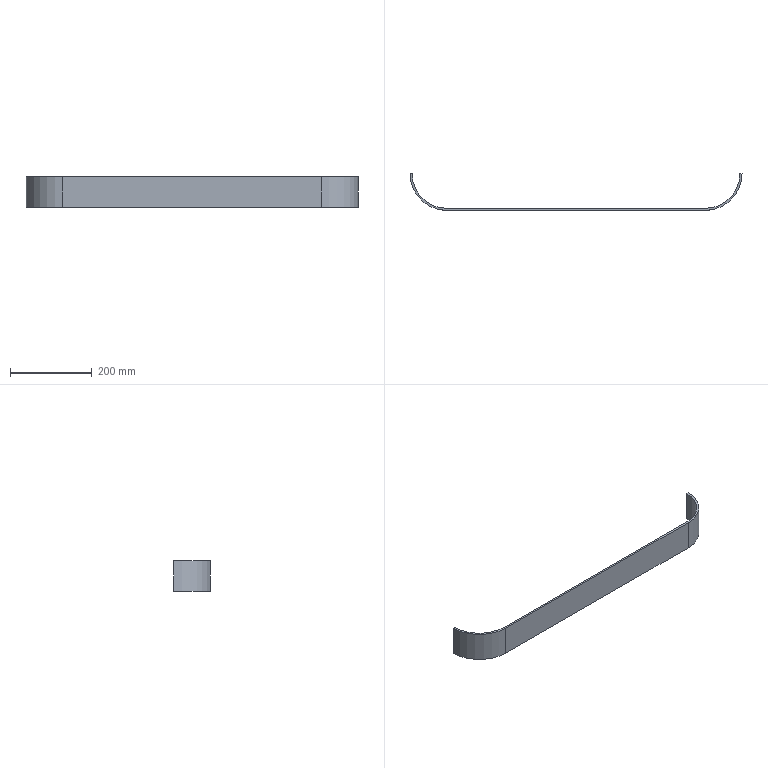Part | NX | features BREP 1 | 1 solid | 10 faces | box 810 x 90 x 75 mm | volume 339334 mm3 | plane 6 | cylinder 4 | commonest cylinder face diameters 170 x2 180 x2
STEP:
#1=CARTESIAN_POINT('',(-315.,0.,75.));
#2=VERTEX_POINT('',#1);
#3=CARTESIAN_POINT('',(-405.,90.,75.));
#4=VERTEX_POINT('',#3);
#5=CARTESIAN_POINT('',(-315.,90.,75.));
#6=DIRECTION('',(0.,0.,-1.));
#7=DIRECTION('',(-1.,0.,0.));
#8=AXIS2_PLACEMENT_3D('',#5,#6,#7);
#9=CIRCLE('',#8,90.);
#10=EDGE_CURVE('',#2,#4,#9,.T.);
#11=ORIENTED_EDGE('',*,*,#10,.F.);
#12=CARTESIAN_POINT('',(315.,0.,75.));
#13=VERTEX_POINT('',#12);
#14=CARTESIAN_POINT('',(-315.,0.,75.));
#15=DIRECTION('',(-1.,0.,0.));
#16=VECTOR('',#15,1000.);
#17=LINE('',#14,#16);
#18=EDGE_CURVE('',#13,#2,#17,.T.);
#19=ORIENTED_EDGE('',*,*,#18,.F.);
#20=CARTESIAN_POINT('',(405.,90.,75.));
#21=VERTEX_POINT('',#20);
#22=CARTESIAN_POINT('',(315.,90.,75.));
#23=DIRECTION('',(0.,0.,-1.));
#24=DIRECTION('',(-1.,0.,0.));
#25=AXIS2_PLACEMENT_3D('',#22,#23,#24);
#26=CIRCLE('',#25,90.);
#27=EDGE_CURVE('',#21,#13,#26,.T.);
#28=ORIENTED_EDGE('',*,*,#27,.F.);
#29=CARTESIAN_POINT('',(400.,90.,75.));
#30=VERTEX_POINT('',#29);
#31=CARTESIAN_POINT('',(400.,90.,75.));
#32=DIRECTION('',(1.,0.,0.));
#33=VECTOR('',#32,1000.);
#34=LINE('',#31,#33);
#35=EDGE_CURVE('',#30,#21,#34,.T.);
#36=ORIENTED_EDGE('',*,*,#35,.F.);
#37=CARTESIAN_POINT('',(315.,5.,75.));
#38=VERTEX_POINT('',#37);
#39=CARTESIAN_POINT('',(315.,90.,75.));
#40=DIRECTION('',(0.,0.,-1.));
#41=DIRECTION('',(1.,0.,0.));
#42=AXIS2_PLACEMENT_3D('',#39,#40,#41);
#43=CIRCLE('',#42,85.);
#44=EDGE_CURVE('',#30,#38,#43,.T.);
#45=ORIENTED_EDGE('',*,*,#44,.T.);
#46=CARTESIAN_POINT('',(-315.,5.,75.));
#47=VERTEX_POINT('',#46);
#48=CARTESIAN_POINT('',(-315.,5.,75.));
#49=DIRECTION('',(-1.,0.,0.));
#50=VECTOR('',#49,1000.);
#51=LINE('',#48,#50);
#52=EDGE_CURVE('',#38,#47,#51,.T.);
#53=ORIENTED_EDGE('',*,*,#52,.T.);
#54=CARTESIAN_POINT('',(-400.,90.,75.));
#55=VERTEX_POINT('',#54);
#56=CARTESIAN_POINT('',(-315.,90.,75.));
#57=DIRECTION('',(0.,0.,-1.));
#58=DIRECTION('',(1.,0.,0.));
#59=AXIS2_PLACEMENT_3D('',#56,#57,#58);
#60=CIRCLE('',#59,85.);
#61=EDGE_CURVE('',#47,#55,#60,.T.);
#62=ORIENTED_EDGE('',*,*,#61,.T.);
#63=CARTESIAN_POINT('',(-405.,90.,75.));
#64=DIRECTION('',(1.,0.,0.));
#65=VECTOR('',#64,1000.);
#66=LINE('',#63,#65);
#67=EDGE_CURVE('',#4,#55,#66,.T.);
#68=ORIENTED_EDGE('',*,*,#67,.F.);
#69=EDGE_LOOP('',(#11,#19,#28,#36,#45,#53,#62,#68));
#70=FACE_BOUND('',#69,.T.);
#71=CARTESIAN_POINT('',(-315.,5.,75.));
#72=DIRECTION('',(0.,0.,1.));
#73=DIRECTION('',(1.,0.,0.));
#74=AXIS2_PLACEMENT_3D('',#71,#72,#73);
#75=PLANE('',#74);
#76=ADVANCED_FACE('',(#70),#75,.T.);
#77=CARTESIAN_POINT('',(-315.,5.,0.));
#78=VERTEX_POINT('',#77);
#79=CARTESIAN_POINT('',(-400.,90.,0.));
#80=VERTEX_POINT('',#79);
#81=CARTESIAN_POINT('',(-315.,90.,0.));
#82=DIRECTION('',(0.,0.,-1.));
#83=DIRECTION('',(1.,0.,0.));
#84=AXIS2_PLACEMENT_3D('',#81,#82,#83);
#85=CIRCLE('',#84,85.);
#86=EDGE_CURVE('',#78,#80,#85,.T.);
#87=ORIENTED_EDGE('',*,*,#86,.F.);
#88=CARTESIAN_POINT('',(315.,5.,0.));
#89=VERTEX_POINT('',#88);
#90=CARTESIAN_POINT('',(-315.,5.,0.));
#91=DIRECTION('',(-1.,0.,0.));
#92=VECTOR('',#91,1000.);
#93=LINE('',#90,#92);
#94=EDGE_CURVE('',#89,#78,#93,.T.);
#95=ORIENTED_EDGE('',*,*,#94,.F.);
#96=CARTESIAN_POINT('',(400.,90.,0.));
#97=VERTEX_POINT('',#96);
#98=CARTESIAN_POINT('',(315.,90.,0.));
#99=DIRECTION('',(0.,0.,-1.));
#100=DIRECTION('',(1.,0.,0.));
#101=AXIS2_PLACEMENT_3D('',#98,#99,#100);
#102=CIRCLE('',#101,85.);
#103=EDGE_CURVE('',#97,#89,#102,.T.);
#104=ORIENTED_EDGE('',*,*,#103,.F.);
#105=CARTESIAN_POINT('',(405.,90.,0.));
#106=VERTEX_POINT('',#105);
#107=CARTESIAN_POINT('',(400.,90.,0.));
#108=DIRECTION('',(1.,0.,0.));
#109=VECTOR('',#108,1000.);
#110=LINE('',#107,#109);
#111=EDGE_CURVE('',#97,#106,#110,.T.);
#112=ORIENTED_EDGE('',*,*,#111,.T.);
#113=CARTESIAN_POINT('',(315.,0.,0.));
#114=VERTEX_POINT('',#113);
#115=CARTESIAN_POINT('',(315.,90.,0.));
#116=DIRECTION('',(0.,0.,-1.));
#117=DIRECTION('',(-1.,0.,0.));
#118=AXIS2_PLACEMENT_3D('',#115,#116,#117);
#119=CIRCLE('',#118,90.);
#120=EDGE_CURVE('',#106,#114,#119,.T.);
#121=ORIENTED_EDGE('',*,*,#120,.T.);
#122=CARTESIAN_POINT('',(-315.,0.,0.));
#123=VERTEX_POINT('',#122);
#124=CARTESIAN_POINT('',(-315.,0.,0.));
#125=DIRECTION('',(-1.,0.,0.));
#126=VECTOR('',#125,1000.);
#127=LINE('',#124,#126);
#128=EDGE_CURVE('',#114,#123,#127,.T.);
#129=ORIENTED_EDGE('',*,*,#128,.T.);
#130=CARTESIAN_POINT('',(-405.,90.,0.));
#131=VERTEX_POINT('',#130);
#132=CARTESIAN_POINT('',(-315.,90.,0.));
#133=DIRECTION('',(0.,0.,-1.));
#134=DIRECTION('',(-1.,0.,0.));
#135=AXIS2_PLACEMENT_3D('',#132,#133,#134);
#136=CIRCLE('',#135,90.);
#137=EDGE_CURVE('',#123,#131,#136,.T.);
#138=ORIENTED_EDGE('',*,*,#137,.T.);
#139=CARTESIAN_POINT('',(-405.,90.,0.));
#140=DIRECTION('',(1.,0.,0.));
#141=VECTOR('',#140,1000.);
#142=LINE('',#139,#141);
#143=EDGE_CURVE('',#131,#80,#142,.T.);
#144=ORIENTED_EDGE('',*,*,#143,.T.);
#145=EDGE_LOOP('',(#87,#95,#104,#112,#121,#129,#138,#144));
#146=FACE_BOUND('',#145,.T.);
#147=CARTESIAN_POINT('',(-315.,0.,0.));
#148=DIRECTION('',(0.,0.,-1.));
#149=DIRECTION('',(-1.,0.,0.));
#150=AXIS2_PLACEMENT_3D('',#147,#148,#149);
#151=PLANE('',#150);
#152=ADVANCED_FACE('',(#146),#151,.T.);
#153=ORIENTED_EDGE('',*,*,#86,.T.);
#154=CARTESIAN_POINT('',(-400.,90.,75.));
#155=DIRECTION('',(0.,0.,-1.));
#156=VECTOR('',#155,1000.);
#157=LINE('',#154,#156);
#158=EDGE_CURVE('',#55,#80,#157,.T.);
#159=ORIENTED_EDGE('',*,*,#158,.F.);
#160=ORIENTED_EDGE('',*,*,#61,.F.);
#161=CARTESIAN_POINT('',(-315.,5.,75.));
#162=DIRECTION('',(0.,0.,-1.));
#163=VECTOR('',#162,1000.);
#164=LINE('',#161,#163);
#165=EDGE_CURVE('',#47,#78,#164,.T.);
#166=ORIENTED_EDGE('',*,*,#165,.T.);
#167=EDGE_LOOP('',(#153,#159,#160,#166));
#168=FACE_BOUND('',#167,.T.);
#169=CARTESIAN_POINT('',(-315.,90.,75.));
#170=DIRECTION('',(0.,0.,-1.));
#171=DIRECTION('',(-1.,0.,0.));
#172=AXIS2_PLACEMENT_3D('',#169,#170,#171);
#173=CYLINDRICAL_SURFACE('',#172,85.);
#174=ADVANCED_FACE('',(#168),#173,.F.);
#175=ORIENTED_EDGE('',*,*,#143,.F.);
#176=CARTESIAN_POINT('',(-405.,90.,75.));
#177=DIRECTION('',(0.,0.,-1.));
#178=VECTOR('',#177,1000.);
#179=LINE('',#176,#178);
#180=EDGE_CURVE('',#4,#131,#179,.T.);
#181=ORIENTED_EDGE('',*,*,#180,.F.);
#182=ORIENTED_EDGE('',*,*,#67,.T.);
#183=ORIENTED_EDGE('',*,*,#158,.T.);
#184=EDGE_LOOP('',(#175,#181,#182,#183));
#185=FACE_BOUND('',#184,.T.);
#186=CARTESIAN_POINT('',(-405.,90.,75.));
#187=DIRECTION('',(0.,1.,0.));
#188=DIRECTION('',(-1.,0.,0.));
#189=AXIS2_PLACEMENT_3D('',#186,#187,#188);
#190=PLANE('',#189);
#191=ADVANCED_FACE('',(#185),#190,.T.);
#192=ORIENTED_EDGE('',*,*,#137,.F.);
#193=CARTESIAN_POINT('',(-315.,0.,75.));
#194=DIRECTION('',(0.,0.,-1.));
#195=VECTOR('',#194,1000.);
#196=LINE('',#193,#195);
#197=EDGE_CURVE('',#2,#123,#196,.T.);
#198=ORIENTED_EDGE('',*,*,#197,.F.);
#199=ORIENTED_EDGE('',*,*,#10,.T.);
#200=ORIENTED_EDGE('',*,*,#180,.T.);
#201=EDGE_LOOP('',(#192,#198,#199,#200));
#202=FACE_BOUND('',#201,.T.);
#203=CARTESIAN_POINT('',(-315.,90.,75.));
#204=DIRECTION('',(0.,0.,-1.));
#205=DIRECTION('',(-1.,0.,0.));
#206=AXIS2_PLACEMENT_3D('',#203,#204,#205);
#207=CYLINDRICAL_SURFACE('',#206,90.);
#208=ADVANCED_FACE('',(#202),#207,.T.);
#209=ORIENTED_EDGE('',*,*,#128,.F.);
#210=CARTESIAN_POINT('',(315.,0.,75.));
#211=DIRECTION('',(0.,0.,-1.));
#212=VECTOR('',#211,1000.);
#213=LINE('',#210,#212);
#214=EDGE_CURVE('',#13,#114,#213,.T.);
#215=ORIENTED_EDGE('',*,*,#214,.F.);
#216=ORIENTED_EDGE('',*,*,#18,.T.);
#217=ORIENTED_EDGE('',*,*,#197,.T.);
#218=EDGE_LOOP('',(#209,#215,#216,#217));
#219=FACE_BOUND('',#218,.T.);
#220=CARTESIAN_POINT('',(-315.,0.,75.));
#221=DIRECTION('',(0.,-1.,0.));
#222=DIRECTION('',(1.,0.,0.));
#223=AXIS2_PLACEMENT_3D('',#220,#221,#222);
#224=PLANE('',#223);
#225=ADVANCED_FACE('',(#219),#224,.T.);
#226=ORIENTED_EDGE('',*,*,#120,.F.);
#227=CARTESIAN_POINT('',(405.,90.,75.));
#228=DIRECTION('',(0.,0.,-1.));
#229=VECTOR('',#228,1000.);
#230=LINE('',#227,#229);
#231=EDGE_CURVE('',#21,#106,#230,.T.);
#232=ORIENTED_EDGE('',*,*,#231,.F.);
#233=ORIENTED_EDGE('',*,*,#27,.T.);
#234=ORIENTED_EDGE('',*,*,#214,.T.);
#235=EDGE_LOOP('',(#226,#232,#233,#234));
#236=FACE_BOUND('',#235,.T.);
#237=CARTESIAN_POINT('',(315.,90.,75.));
#238=DIRECTION('',(0.,0.,-1.));
#239=DIRECTION('',(-1.,0.,0.));
#240=AXIS2_PLACEMENT_3D('',#237,#238,#239);
#241=CYLINDRICAL_SURFACE('',#240,90.);
#242=ADVANCED_FACE('',(#236),#241,.T.);
#243=ORIENTED_EDGE('',*,*,#111,.F.);
#244=CARTESIAN_POINT('',(400.,90.,75.));
#245=DIRECTION('',(0.,0.,-1.));
#246=VECTOR('',#245,1000.);
#247=LINE('',#244,#246);
#248=EDGE_CURVE('',#30,#97,#247,.T.);
#249=ORIENTED_EDGE('',*,*,#248,.F.);
#250=ORIENTED_EDGE('',*,*,#35,.T.);
#251=ORIENTED_EDGE('',*,*,#231,.T.);
#252=EDGE_LOOP('',(#243,#249,#250,#251));
#253=FACE_BOUND('',#252,.T.);
#254=CARTESIAN_POINT('',(400.,90.,75.));
#255=DIRECTION('',(0.,1.,0.));
#256=DIRECTION('',(-1.,0.,0.));
#257=AXIS2_PLACEMENT_3D('',#254,#255,#256);
#258=PLANE('',#257);
#259=ADVANCED_FACE('',(#253),#258,.T.);
#260=ORIENTED_EDGE('',*,*,#103,.T.);
#261=CARTESIAN_POINT('',(315.,5.,75.));
#262=DIRECTION('',(0.,0.,-1.));
#263=VECTOR('',#262,1000.);
#264=LINE('',#261,#263);
#265=EDGE_CURVE('',#38,#89,#264,.T.);
#266=ORIENTED_EDGE('',*,*,#265,.F.);
#267=ORIENTED_EDGE('',*,*,#44,.F.);
#268=ORIENTED_EDGE('',*,*,#248,.T.);
#269=EDGE_LOOP('',(#260,#266,#267,#268));
#270=FACE_BOUND('',#269,.T.);
#271=CARTESIAN_POINT('',(315.,90.,75.));
#272=DIRECTION('',(0.,0.,-1.));
#273=DIRECTION('',(-1.,0.,0.));
#274=AXIS2_PLACEMENT_3D('',#271,#272,#273);
#275=CYLINDRICAL_SURFACE('',#274,85.);
#276=ADVANCED_FACE('',(#270),#275,.F.);
#277=ORIENTED_EDGE('',*,*,#94,.T.);
#278=ORIENTED_EDGE('',*,*,#165,.F.);
#279=ORIENTED_EDGE('',*,*,#52,.F.);
#280=ORIENTED_EDGE('',*,*,#265,.T.);
#281=EDGE_LOOP('',(#277,#278,#279,#280));
#282=FACE_BOUND('',#281,.T.);
#283=CARTESIAN_POINT('',(-315.,5.,75.));
#284=DIRECTION('',(0.,-1.,0.));
#285=DIRECTION('',(1.,0.,0.));
#286=AXIS2_PLACEMENT_3D('',#283,#284,#285);
#287=PLANE('',#286);
#288=ADVANCED_FACE('',(#282),#287,.F.);
#289=CLOSED_SHELL('',(#76,#152,#174,#191,#208,#225,#242,#259,#276,#288));
#290=MANIFOLD_SOLID_BREP('',#289);
#291=(LENGTH_UNIT()NAMED_UNIT(*)SI_UNIT(.MILLI.,.METRE.));
#292=UNCERTAINTY_MEASURE_WITH_UNIT(LENGTH_MEASURE(0.00001),#291,'','');
#293=(NAMED_UNIT(*)PLANE_ANGLE_UNIT()SI_UNIT($,.RADIAN.));
#294=(NAMED_UNIT(*)SI_UNIT($,.STERADIAN.)SOLID_ANGLE_UNIT());
#295=(GEOMETRIC_REPRESENTATION_CONTEXT(3)GLOBAL_UNCERTAINTY_ASSIGNED_CONTEXT((#292))GLOBAL_UNIT_ASSIGNED_CONTEXT((#291,#293,#294))REPRESENTATION_CONTEXT('',''));
#296=ADVANCED_BREP_SHAPE_REPRESENTATION('',(#290),#295);